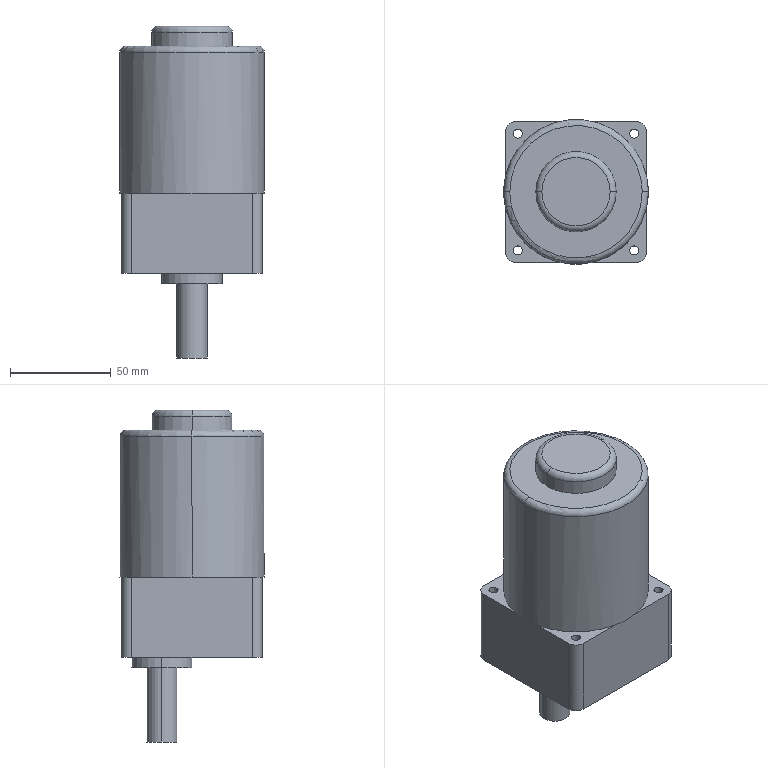Part | STEP file | M8IA15_default | 1 solid | 41 faces | box 71.8 x 71.8 x 165 mm | volume 514049 mm3 | cylinder 20 | plane 17 | torus 4 | commonest cylinder face diameters 4.5 x8 10 x4 15 x2 30 x2 40 x2 71.8 x2